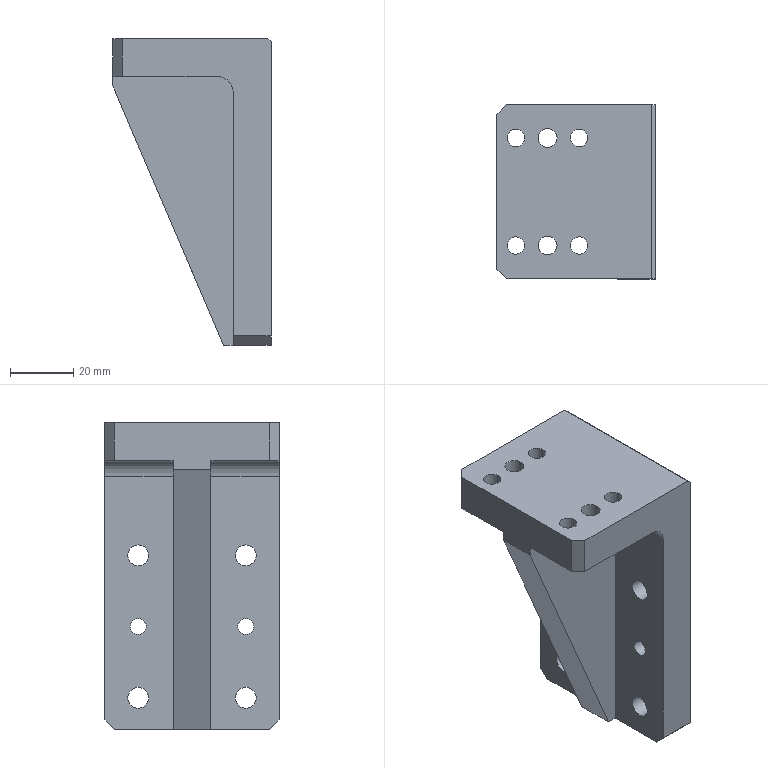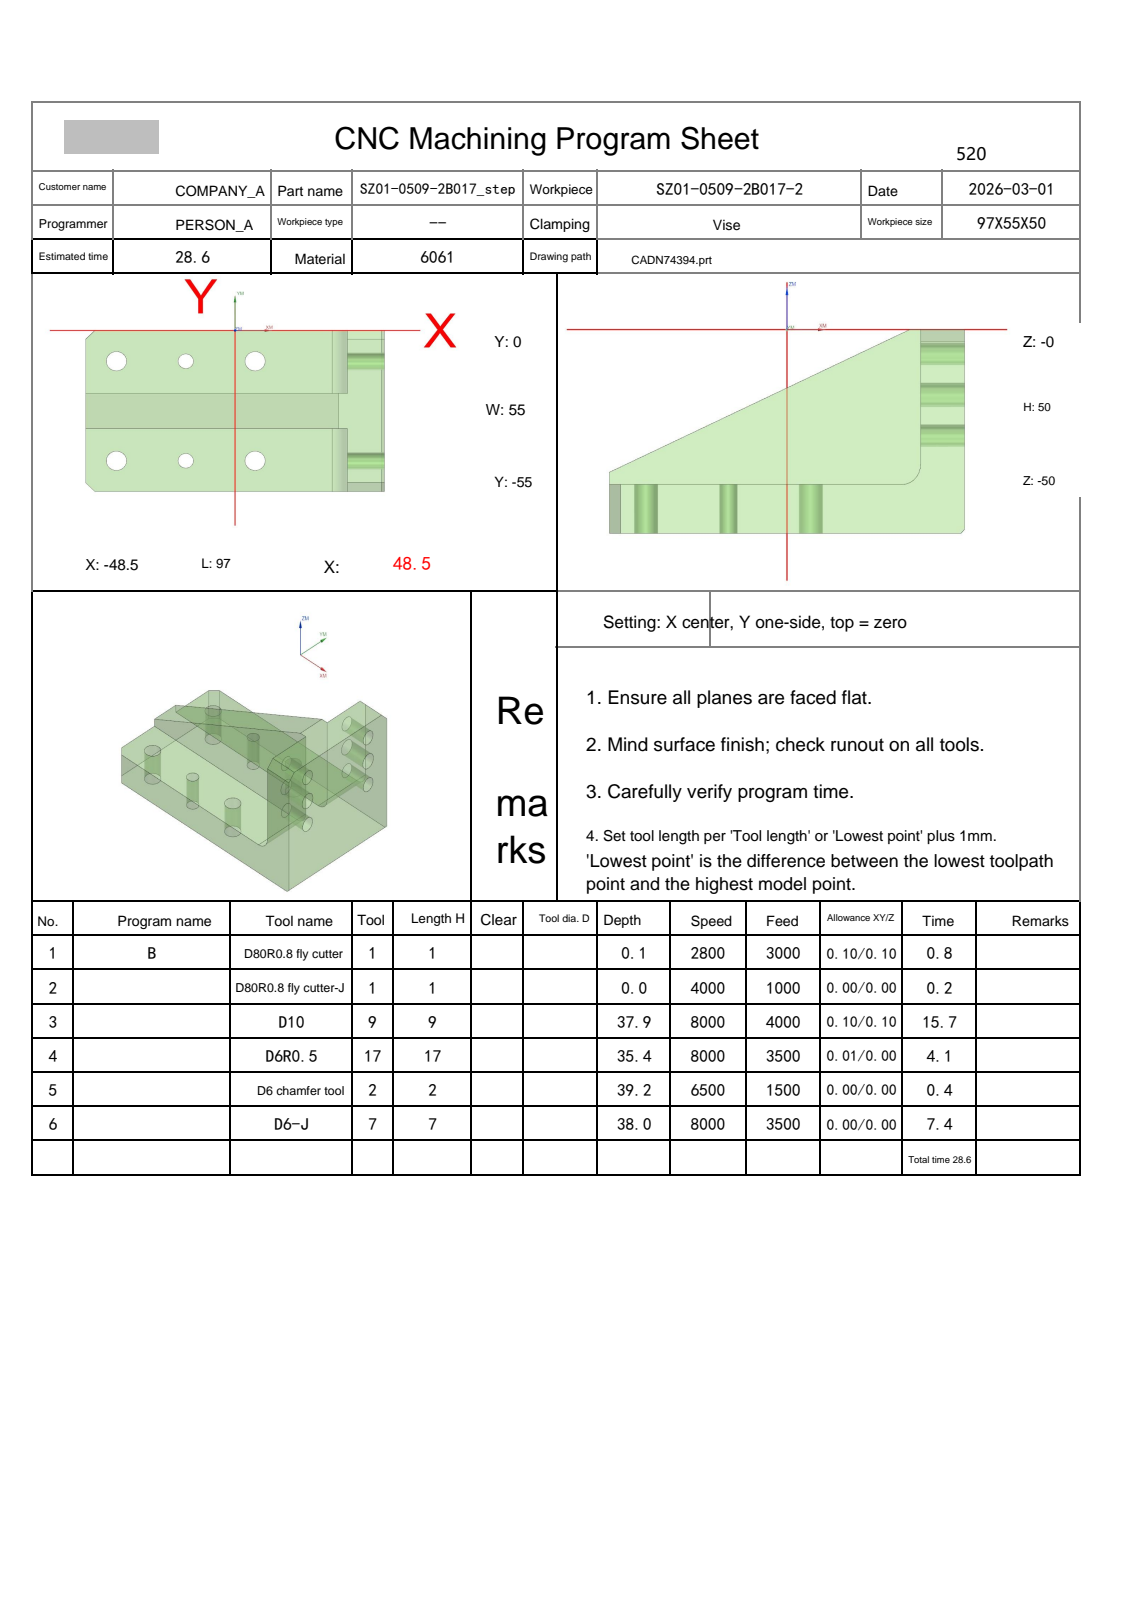NC program | NX | posted by the shop | part box 50 x 55 x 97 mm
Lines 110 to 1246 of 18128:
N3 T09 M06
(D10  D=10. R=0. H=09 ce=0.10 di=0.10)
G00 G90 G54 X-4.751 Y-69.5 M03 S8000
G43 H09 Z14.5
M08
Z.701
G01 Z-.499 F4000.
Y-62.08
G03 X-11.751 Y-55.08 I-7. J0.0
G01 X-45.5
X-45.557 Y-55.057
X-48.557 Y-52.057
X-48.58 Y-52.
Y-38.678
G02 X-50.965 Y-38.008 I.232 J5.41
X-51.5 Y-37.642 I2.818 J4.689
G01 Y-17.385
G02 X-48.58 Y-16.325 I3.189 J-4.232
G01 Y-3.
X-48.557 Y-2.943
X-45.557 Y.057
X-45.5 Y.08
X31.301
X31.324 Y.09
X31.362 Y.651
G02 X32.353 Y3. I5.275 J-.842
G01 X32.988
G02 X36.5 Y4.04 I3.533 J-5.481
G01 X48.42
Y3.
X48.5
X48.504 Y4.04
X48.501 Y3.
X48.58
Y2.64
X48.501
X48.5 Y2.641
X48.499 Y2.64
X48.42 Y2.641
X36.5 Y2.64
G03 X31.424 Y-1.987 I.021 J-5.121
G01 X31.379 Y-2.26
X31.344 Y-2.498
X31.321 Y-2.991
X31.32 Y-3.243
X31.321 Y-3.438
X31.32 Y-16.494
G03 X27.077 Y-21.5 I.856 J-5.027
G01 Y-33.5
G03 X31.322 Y-38.506 I5.1 J.022
G01 X31.321 Y-51.562
Y-52.069
X31.345 Y-52.51
X31.424 Y-53.011
G03 X36.5 Y-57.64 I5.097 J.491
G01 X48.42
X48.499
X48.5 Y-57.641
X48.501 Y-57.64
X48.58
Y-58.
X48.502
X48.506 Y-59.04
X48.5
Y-58.
X48.42
Y-59.04
X36.494
G02 X32.988 Y-58. I.026 J6.521
G01 X32.301
G02 X31.32 Y-55.082 I4.155 J3.02
G01 X30.524 Y-55.081
X26.802 Y-55.08
X25.909
X-8.737
G02 X-9.55 Y-54.662 I.001 J1.
G01 X-13.952 Y-48.498
G03 X-14.765 Y-48.08 I-.813 J-.582
G01 X-40.582
G02 X-41.58 Y-47.082 I.002 J1.
G01 Y-38.678
G03 X-44.136 Y-33.269 I-7. J0.0
G02 X-44.5 Y-32.5 I.636 J.771
G01 Y-22.503
G02 X-44.136 Y-21.734 I1. J-.002
G03 X-41.58 Y-16.325 I-4.444 J5.409
G01 Y-7.918
G02 X-40.582 Y-6.92 I1. J-.002
G01 X23.323
G02 X24.321 Y-7.918 I-.002 J-1.
G01 Y-11.871
G02 X23.998 Y-12.605 I-1. J.002
G03 X20.077 Y-21.485 I8.179 J-8.917
G01 Y-33.515
G03 X23.999 Y-42.396 I12.1 J.037
G02 X24.322 Y-43.13 I-.677 J-.736
G01 Y-47.082
G02 X23.324 Y-48.08 I-1. J.002
G01 X-8.737
G02 X-9.55 Y-47.662 I0.0 J1.
G01 X-13.952 Y-41.498
G03 X-14.765 Y-41.08 I-.814 J-.582
G01 X-33.582
G02 X-34.58 Y-40.082 I.002 J1.
G01 Y-38.678
G03 X-37.307 Y-30.376 I-14. J0.0
G02 X-37.5 Y-29.788 I.807 J.591
G01 Y-25.215
G02 X-37.307 Y-24.626 I1. J-.002
G03 X-34.58 Y-16.325 I-11.273 J8.301
G01 Y-14.918
G02 X-33.582 Y-13.92 I1. J-.002
G01 X13.194
G02 X14.192 Y-14.92 I-.002 J-1.
X14.137 Y-15.247 I-1. J0.0
G03 X13.077 Y-21.474 I18.039 J-6.275
G01 Y-33.526
G03 X14.137 Y-39.754 I19.1 J.047
G02 X14.192 Y-40.08 I-.945 J-.326
X13.194 Y-41.08 I-1. J0.0
G01 X-8.737
G02 X-9.55 Y-40.662 I0.0 J1.
G01 X-13.952 Y-34.498
G03 X-14.765 Y-34.08 I-.814 J-.582
G01 X-27.307
G02 X-28.27 Y-33.337 I.003 J1.
G03 X-30.368 Y-28.221 I-20.31 J-5.341
G02 X-30.5 Y-27.728 I.869 J.496
G01 Y-27.275
G02 X-30.368 Y-26.782 I1. J-.003
G03 X-28.27 Y-21.663 I-18.212 J10.457
G02 X-27.306 Y-20.92 I.966 J-.257
G01 X5.08
G02 X6.077 Y-21.918 I-.003 J-1.
G01 Y-33.083
G02 X5.08 Y-34.08 I-1. J.003
G01 X-9.087
G02 X-9.794 Y-33.787 I0.0 J1.
G01 X-13.708 Y-29.873
G03 X-14.415 Y-29.58 I-.707 J-.707
G01 X-24.082
G02 X-25.003 Y-28.964 I.003 J1.
G03 X-25.46 Y-27.921 I-23.577 J-9.714
G02 X-25.552 Y-27.501 I.908 J.419
X-25.46 Y-27.082 I1. J0.0
G03 X-25.002 Y-26.037 I-23.12 J10.757
G02 X-24.081 Y-25.42 I.924 J-.383
G01 X.58
G02 X1.577 Y-26.417 I-.003 J-1.
G01 Y-28.583
G02 X.58 Y-29.58 I-1. J.003
G01 X-11.751
X-12.251
G03 X-19.251 Y-36.58 I0.0 J-7.
G01 Z.701
G00 Z3.
G01 X-4.751 Y-69.5 F6000.
G00 Z.203
G01 Z-.997 F4000.
Y-62.08
G03 X-11.751 Y-55.08 I-7. J0.0
G01 X-45.5
X-45.557 Y-55.057
X-48.557 Y-52.057
X-48.58 Y-52.
Y-38.678
G02 X-50.965 Y-38.008 I.232 J5.41
X-53.609 Y-33.631 I2.818 J4.689
G01 Y-21.36
X-53.545 Y-20.788
G02 X-48.58 Y-16.325 I5.234 J-.83
G01 Y-3.
X-48.557 Y-2.943
X-45.557 Y.057
X-45.5 Y.08
X31.301
X31.324 Y.09
X31.362 Y.651
G02 X36.629 Y5.151 I5.275 J-.842
G01 X48.501
X48.585 Y5.156
X48.581 Y5.071
X48.58 Y3.139
X48.5
X48.42
X36.5
G03 X31.398 Y-1.984 I.021 J-5.122
G01 X31.4 Y-2.119
X31.344 Y-2.498
X31.321 Y-2.991
X31.32 Y-3.243
X31.321 Y-3.438
X31.32 Y-16.4
X31.163
X31.09 Y-16.399
G03 X25.909 Y-21.5 I0.0 J-5.183
G01 Y-33.5
G03 X31.09 Y-38.601 I5.182 J.082
G01 X31.163 Y-38.6
X31.322
X31.321 Y-51.562
Y-52.069
X31.345 Y-52.51
X31.4 Y-52.879
Y-52.997
Y-53.018
G03 X36.5 Y-58.139 I5.121 J0.0
G01 X48.42
X48.5
X48.58
X48.581 Y-60.071
X48.585 Y-60.156
X48.501 Y-60.151
X36.623 Y-60.15
X35.717 Y-60.071
X34.817 Y-59.849
G02 X31.32 Y-55.082 I1.639 J4.868
G01 X26.802 Y-55.08
X25.909
X-8.737
G02 X-9.55 Y-54.662 I.001 J1.
G01 X-13.952 Y-48.498
G03 X-14.765 Y-48.08 I-.813 J-.582
G01 X-40.582
G02 X-41.58 Y-47.082 I.002 J1.
G01 Y-38.678
G03 X-45.982 Y-32.178 I-7. J0.0
G02 X-46.609 Y-31.251 I.373 J.928
G01 Y-23.751
G02 X-45.982 Y-22.825 I1. J-.002
G03 X-41.58 Y-16.325 I-2.598 J6.5
G01 Y-7.918
G02 X-40.582 Y-6.92 I1. J-.002
G01 X23.322
G02 X24.321 Y-7.919 I-.002 J-1.
G01 Y-10.934
G02 X23.911 Y-11.74 I-1. J.002
G03 X18.909 Y-21.445 I7.179 J-9.842
G01 Y-33.555
G03 X23.912 Y-43.261 I12.182 J.138
G02 X24.322 Y-44.067 I-.591 J-.807
G01 Y-47.082
G02 X23.323 Y-48.08 I-1. J.002
G01 X-8.737
G02 X-9.55 Y-47.662 I0.0 J1.
G01 X-13.952 Y-41.498
G03 X-14.765 Y-41.08 I-.814 J-.582
G01 X-33.582
G02 X-34.58 Y-40.082 I.002 J1.
G01 Y-38.678
G03 X-39.244 Y-28.245 I-14. J0.0
G02 X-39.576 Y-27.501 I.668 J.744
X-39.244 Y-26.757 I1. J0.0
G03 X-34.58 Y-16.325 I-9.336 J10.433
G01 Y-14.918
G02 X-33.582 Y-13.92 I1. J-.002
G01 X12.041
G02 X13.039 Y-14.92 I-.002 J-1.
X12.984 Y-15.249 I-1. J0.0
G03 X11.909 Y-21.365 I18.107 J-6.334
G01 Y-33.634
G03 X12.984 Y-39.752 I19.181 J.217
G02 X13.039 Y-40.08 I-.945 J-.328
X12.041 Y-41.08 I-1. J0.0
G01 X-8.737
G02 X-9.55 Y-40.662 I0.0 J1.
G01 X-13.952 Y-34.498
G03 X-14.765 Y-34.08 I-.814 J-.582
G01 X-27.306
G02 X-28.271 Y-33.337 I.002 J1.
G03 X-30.493 Y-28.007 I-20.309 J-5.341
G02 X-30.63 Y-27.501 I.863 J.506
X-30.493 Y-26.995 I1. J0.0
G03 X-28.27 Y-21.664 I-18.087 J10.67
G02 X-27.306 Y-20.92 I.967 J-.257
G01 X3.911
G02 X4.909 Y-21.918 I-.002 J-1.
G01 Y-33.082
G02 X3.911 Y-34.08 I-1. J.002
G01 X-9.087
G02 X-9.794 Y-33.787 I0.0 J1.
G01 X-13.708 Y-29.873
G03 X-14.415 Y-29.58 I-.707 J-.707
G01 X-24.082
G02 X-25.003 Y-28.963 I.003 J1.
G03 X-25.46 Y-27.921 I-23.577 J-9.714
G02 X-25.552 Y-27.501 I.908 J.419
X-25.46 Y-27.082 I1. J0.0
G03 X-25.002 Y-26.037 I-23.12 J10.757
G02 X-24.081 Y-25.42 I.924 J-.383
G01 X-.588
G02 X.409 Y-26.418 I-.003 J-1.
G01 Y-28.583
G02 X-.588 Y-29.58 I-1. J.003
G01 X-11.751
X-12.251
G03 X-19.251 Y-36.58 I0.0 J-7.
G01 Z.203
G00 Z3.
G01 X-4.751 Y-69.5 F6000.
G00 Z-.296
G01 Z-1.496 F4000.
Y-62.08
G03 X-11.751 Y-55.08 I-7. J0.0
G01 X-45.5
X-45.557 Y-55.057
X-48.557 Y-52.057
X-48.58 Y-52.
Y-38.678
G02 X-50.965 Y-38.008 I.232 J5.41
X-53.609 Y-33.631 I2.818 J4.689
G01 Y-21.36
X-53.545 Y-20.788
G02 X-48.58 Y-16.325 I5.234 J-.83
G01 Y-3.
X-48.557 Y-2.943
X-45.557 Y.057
X-45.5 Y.08
X31.301
X31.324 Y.09
X31.362 Y.651
G02 X36.629 Y5.151 I5.275 J-.842
G01 X48.501
X48.585 Y5.156
X48.581 Y5.071
X48.58 Y3.637
X48.5
X48.42
X36.5
G03 X31.4 Y-1.483 I.021 J-5.121
G01 Y-1.504
Y-2.119
X31.344 Y-2.498
X31.321 Y-2.991
X31.32 Y-3.243
X31.321 Y-3.438
X31.32 Y-16.4
X29.995
X29.925
G03 X24.74 Y-21.5 I0.0 J-5.185
G01 Y-33.5
G03 X29.925 Y-38.6 I5.185 J.085
G01 X29.995
X31.018
X31.163
X31.322
X31.321 Y-51.562
Y-52.069
X31.345 Y-52.51
X31.4 Y-52.879
Y-53.496
Y-53.517
G03 X36.5 Y-58.637 I5.121 J0.0
G01 X48.42
X48.499
X48.58
X48.581 Y-60.071
X48.585 Y-60.156
X48.501 Y-60.151
X36.623 Y-60.15
X35.717 Y-60.071
X34.817 Y-59.849
G02 X31.32 Y-55.082 I1.639 J4.868
G01 X26.802 Y-55.08
X25.909
X-8.737
G02 X-9.55 Y-54.662 I0.0 J1.
G01 X-13.952 Y-48.498
G03 X-14.765 Y-48.08 I-.813 J-.582
G01 X-40.582
G02 X-41.58 Y-47.082 I.002 J1.
G01 Y-38.678
G03 X-45.982 Y-32.178 I-7. J0.0
G02 X-46.609 Y-31.251 I.373 J.928
G01 Y-23.751
G02 X-45.982 Y-22.825 I1. J-.002
G03 X-41.58 Y-16.325 I-2.598 J6.5
G01 Y-7.918
G02 X-40.582 Y-6.92 I1. J-.002
G01 X23.323
G02 X24.321 Y-7.919 I-.002 J-1.
G01 Y-10.175
G02 X23.823 Y-11.037 I-1. J.002
G03 X17.74 Y-21.443 I6.102 J-10.548
G01 Y-33.557
G03 X23.824 Y-43.963 I12.185 J.143
G02 X24.322 Y-44.826 I-.502 J-.865
G01 Y-47.082
G02 X23.323 Y-48.08 I-1. J.002
G01 X-8.737
G02 X-9.55 Y-47.662 I0.0 J1.
G01 X-13.952 Y-41.498
G03 X-14.765 Y-41.08 I-.814 J-.582
G01 X-33.582
G02 X-34.58 Y-40.082 I.002 J1.
G01 Y-38.678
G03 X-39.244 Y-28.245 I-14. J0.0
G02 X-39.576 Y-27.501 I.668 J.744
X-39.244 Y-26.758 I1. J0.0
G03 X-34.58 Y-16.325 I-9.336 J10.433
G01 Y-14.918
G02 X-33.582 Y-13.92 I1. J-.002
G01 X10.874
G02 X11.871 Y-14.92 I-.002 J-1.
X11.816 Y-15.249 I-1. J0.0
G03 X10.74 Y-21.402 I18.109 J-6.337
G01 Y-33.598
G03 X11.816 Y-39.752 I19.185 J.184
G02 X11.872 Y-40.08 I-.945 J-.328
X10.874 Y-41.08 I-1. J0.0
G01 X-8.737
G02 X-9.55 Y-40.662 I0.0 J1.
G01 X-13.952 Y-34.498
G03 X-14.765 Y-34.08 I-.814 J-.582
G01 X-27.306
G02 X-28.271 Y-33.337 I.002 J1.
G03 X-30.493 Y-28.007 I-20.309 J-5.341
G02 X-30.63 Y-27.501 I.863 J.506
X-30.493 Y-26.995 I1. J0.0
G03 X-28.27 Y-21.663 I-18.087 J10.67
G02 X-27.306 Y-20.92 I.967 J-.257
G01 X2.743
G02 X3.74 Y-21.918 I-.002 J-1.
G01 Y-33.082
G02 X2.743 Y-34.08 I-1. J.002
G01 X-9.087
G02 X-9.794 Y-33.787 I0.0 J1.
G01 X-13.708 Y-29.873
G03 X-14.415 Y-29.58 I-.707 J-.707
G01 X-24.082
G02 X-25.003 Y-28.963 I.003 J1.
G03 X-25.46 Y-27.921 I-23.577 J-9.714
G02 X-25.552 Y-27.501 I.908 J.419
X-25.46 Y-27.082 I1. J0.0
G03 X-25.002 Y-26.037 I-23.12 J10.757
G02 X-24.081 Y-25.42 I.924 J-.383
G01 X-1.757
G02 X-.76 Y-26.418 I-.003 J-1.
G01 Y-28.583
G02 X-1.757 Y-29.58 I-1. J.003
G01 X-11.751
X-12.251
G03 X-19.251 Y-36.58 I0.0 J-7.
G01 Z-.296
G00 Z3.
G01 X-4.751 Y-69.5 F6000.
G00 Z-.795
G01 Z-1.995 F4000.
Y-62.08
G03 X-11.751 Y-55.08 I-7. J0.0
G01 X-45.5
X-45.557 Y-55.057
X-48.557 Y-52.057
X-48.58 Y-52.
Y-38.678
G02 X-50.965 Y-38.008 I.232 J5.41
X-53.609 Y-33.631 I2.818 J4.689
G01 Y-21.36
X-53.545 Y-20.788
G02 X-48.58 Y-16.325 I5.234 J-.83
G01 Y-3.
X-48.557 Y-2.943
X-45.557 Y.057
X-45.5 Y.08
X31.301
X31.324 Y.09
X31.362 Y.651
G02 X36.629 Y5.151 I5.275 J-.842
G01 X48.501
X48.585 Y5.156
X48.581 Y5.071
X48.58 Y4.136
X48.5
X48.496
X48.42
X36.5
G03 X31.4 Y-.985 I.021 J-5.121
G01 Y-1.005
Y-2.119
X31.344 Y-2.498
X31.321 Y-2.991
X31.32 Y-3.243
X31.321 Y-3.438
X31.32 Y-16.4
X29.995
X29.855
X28.827
X28.749 Y-16.399
G03 X23.572 Y-21.5 I0.0 J-5.178
G01 Y-33.5
G03 X28.749 Y-38.601 I5.177 J.077
G01 X28.827 Y-38.6
X31.322
X31.321 Y-51.562
Y-52.069
X31.345 Y-52.51
X31.4 Y-52.879
Y-53.995
Y-54.015
G03 X36.5 Y-59.136 I5.121 J0.0
G01 X48.42
X48.496
X48.5
X48.58
X48.581 Y-60.071
X48.585 Y-60.156
X48.501 Y-60.151
X36.623 Y-60.15
X35.717 Y-60.071
X34.817 Y-59.849
G02 X31.32 Y-55.082 I1.639 J4.868
G01 X26.802 Y-55.08
X25.909
X-8.737
G02 X-9.55 Y-54.662 I.001 J1.
G01 X-13.952 Y-48.498
G03 X-14.765 Y-48.08 I-.813 J-.582
G01 X-40.582
G02 X-41.58 Y-47.082 I.002 J1.
G01 Y-38.678
G03 X-45.982 Y-32.178 I-7. J0.0
G02 X-46.609 Y-31.252 I.373 J.928
G01 Y-23.751
G02 X-45.982 Y-22.825 I1. J-.002
G03 X-41.58 Y-16.325 I-2.598 J6.5
G01 Y-7.918
G02 X-40.582 Y-6.92 I1. J-.002
G01 X23.323
G02 X24.321 Y-7.919 I-.002 J-1.
G01 Y-9.571
G02 X23.734 Y-10.48 I-1. J.002
G03 X16.572 Y-21.448 I5.015 J-11.097
G01 Y-33.552
G03 X23.735 Y-44.52 I12.177 J.13
G02 X24.322 Y-45.429 I-.414 J-.91
G01 Y-47.082
G02 X23.323 Y-48.08 I-1. J.002
G01 X-8.737
G02 X-9.55 Y-47.662 I0.0 J1.
G01 X-13.952 Y-41.498
G03 X-14.765 Y-41.08 I-.813 J-.582
G01 X-33.582
G02 X-34.58 Y-40.082 I.002 J1.
G01 Y-38.678
G03 X-39.244 Y-28.245 I-14. J0.0
G02 X-39.576 Y-27.501 I.669 J.744
X-39.244 Y-26.758 I1. J0.0
G03 X-34.58 Y-16.325 I-9.336 J10.433
G01 Y-14.918
G02 X-33.582 Y-13.92 I1. J-.002
G01 X9.703
G02 X10.701 Y-14.92 I-.002 J-1.
X10.646 Y-15.248 I-1. J0.0
G03 X9.572 Y-21.373 I18.103 J-6.329
G01 Y-33.627
G03 X10.646 Y-39.752 I19.177 J.204
G02 X10.701 Y-40.08 I-.945 J-.328
X9.703 Y-41.08 I-1. J0.0
G01 X-8.737
G02 X-9.55 Y-40.662 I0.0 J1.
G01 X-13.952 Y-34.498
G03 X-14.765 Y-34.08 I-.814 J-.582
G01 X-27.307
G02 X-28.271 Y-33.337 I.003 J1.
G03 X-30.493 Y-28.007 I-20.309 J-5.341
G02 X-30.63 Y-27.501 I.863 J.506
X-30.493 Y-26.995 I1. J0.0
G03 X-28.27 Y-21.663 I-18.087 J10.671
G02 X-27.306 Y-20.92 I.966 J-.257
G01 X1.575
G02 X2.572 Y-21.918 I-.003 J-1.
G01 Y-33.083
G02 X1.575 Y-34.08 I-1. J.003
G01 X-9.087
G02 X-9.794 Y-33.787 I0.0 J1.
G01 X-13.708 Y-29.873
G03 X-14.415 Y-29.58 I-.707 J-.707
G01 X-24.082
G02 X-25.003 Y-28.963 I.003 J1.
G03 X-25.46 Y-27.921 I-23.577 J-9.714
G02 X-25.552 Y-27.501 I.908 J.419
X-25.46 Y-27.082 I1. J0.0
G03 X-25.002 Y-26.037 I-23.12 J10.757
G02 X-24.081 Y-25.42 I.924 J-.383
G01 X-2.925
G02 X-1.928 Y-26.418 I-.003 J-1.
G01 Y-28.583
G02 X-2.925 Y-29.58 I-1. J.003
G01 X-11.751
X-12.251
G03 X-19.251 Y-36.58 I0.0 J-7.
G01 Z-.795
G00 Z3.
G01 X-4.751 Y-69.5 F6000.
G00 Z-1.293
G01 Z-2.493 F4000.
Y-62.08
G03 X-11.751 Y-55.08 I-7. J0.0
G01 X-45.5
X-45.557 Y-55.057
X-48.557 Y-52.057
X-48.58 Y-52.
Y-38.678
G02 X-50.965 Y-38.008 I.232 J5.41
X-53.609 Y-33.631 I2.818 J4.689
G01 Y-21.36
X-53.545 Y-20.788
G02 X-48.58 Y-16.325 I5.234 J-.83
G01 Y-3.
X-48.557 Y-2.943
X-45.557 Y.057
X-45.5 Y.08
X31.301
X31.324 Y.09
X31.362 Y.651
G02 X36.629 Y5.151 I5.275 J-.842
G01 X48.501
X48.585 Y5.156
X48.581 Y5.071
X48.58 Y4.635
X48.5
X48.491
X48.42
X36.5
G03 X31.4 Y-.486 I.021 J-5.121
G01 Y-.507
Y-2.119
X31.344 Y-2.498
X31.321 Y-2.991
X31.32 Y-3.243
X31.321 Y-3.438
X31.32 Y-16.4
X27.658
X27.581 Y-16.399
G03 X22.404 Y-21.5 I0.0 J-5.178
G01 Y-33.5
G03 X27.581 Y-38.601 I5.177 J.077
G01 X27.658 Y-38.6
X28.672
X28.827
X31.322
X31.321 Y-51.562
Y-52.069
X31.345 Y-52.51
X31.4 Y-52.879
Y-54.493
Y-54.514
G03 X36.5 Y-59.635 I5.121 J0.0
G01 X48.42
X48.483
X48.5
X48.58
X48.581 Y-60.071
X48.585 Y-60.156
X48.501 Y-60.151
X36.623 Y-60.15
X35.717 Y-60.071
X34.817 Y-59.849
G02 X31.32 Y-55.082 I1.639 J4.868
G01 X26.802 Y-55.08
X25.909
X-8.737
G02 X-9.55 Y-54.662 I0.0 J1.
G01 X-13.952 Y-48.498
G03 X-14.765 Y-48.08 I-.813 J-.582
G01 X-40.582
G02 X-41.58 Y-47.082 I.002 J1.
G01 Y-38.678
G03 X-45.982 Y-32.178 I-7. J0.0
G02 X-46.609 Y-31.252 I.373 J.928
G01 Y-23.751
G02 X-45.982 Y-22.825 I1. J-.002
G03 X-41.58 Y-16.325 I-2.598 J6.5
G01 Y-7.918
G02 X-40.582 Y-6.92 I1. J-.002
G01 X23.323
G02 X24.321 Y-7.918 I-.002 J-1.
G01 Y-9.109
G02 X23.646 Y-10.053 I-1. J.002
G03 X15.404 Y-21.448 I3.935 J-11.525
G01 Y-33.605
G03 X23.647 Y-44.948 I12.177 J.182
G02 X24.322 Y-45.891 I-.325 J-.946
G01 Y-47.082
G02 X23.324 Y-48.08 I-1. J.002
G01 X-8.737
G02 X-9.55 Y-47.662 I0.0 J1.
G01 X-13.952 Y-41.498
G03 X-14.765 Y-41.08 I-.814 J-.582
G01 X-33.582
G02 X-34.58 Y-40.082 I.002 J1.
G01 Y-38.678
G03 X-39.244 Y-28.245 I-14. J0.0
G02 X-39.576 Y-27.501 I.669 J.744
X-39.244 Y-26.758 I1. J0.0
G03 X-34.58 Y-16.325 I-9.336 J10.433
G01 Y-14.918
G02 X-33.582 Y-13.92 I1. J-.002
G01 X8.535
G02 X9.533 Y-14.92 I-.002 J-1.
X9.477 Y-15.248 I-1. J0.0
G03 X8.404 Y-21.411 I18.103 J-6.33
G01 X8.405 Y-33.709
G03 X9.478 Y-39.752 I19.176 J.287
G02 X9.533 Y-40.08 I-.945 J-.328
X8.535 Y-41.08 I-1. J0.0
G01 X-8.737
G02 X-9.55 Y-40.662 I0.0 J1.
G01 X-13.952 Y-34.498
G03 X-14.765 Y-34.08 I-.814 J-.582
G01 X-27.307
G02 X-28.27 Y-33.337 I.003 J1.
G03 X-30.493 Y-28.007 I-20.31 J-5.341
G02 X-30.63 Y-27.501 I.863 J.506
X-30.493 Y-26.996 I1. J0.0
G03 X-28.27 Y-21.663 I-18.087 J10.671
G02 X-27.306 Y-20.92 I.966 J-.257
G01 X.406
G02 X1.404 Y-21.917 I-.003 J-1.
G01 X1.405 Y-33.083
G02 X.408 Y-34.08 I-1. J.003
G01 X-9.087
G02 X-9.794 Y-33.787 I0.0 J1.
G01 X-13.708 Y-29.873
G03 X-14.415 Y-29.58 I-.707 J-.707
G01 X-24.082
G02 X-25.003 Y-28.964 I.003 J1.
G03 X-25.46 Y-27.921 I-23.577 J-9.714
G02 X-25.552 Y-27.501 I.908 J.419
X-25.46 Y-27.082 I1. J0.0
G03 X-25.002 Y-26.037 I-23.12 J10.757
G02 X-24.081 Y-25.42 I.924 J-.383
G01 X-4.093
G02 X-3.096 Y-26.417 I-.003 J-1.
G01 Y-28.583
G02 X-4.093 Y-29.58 I-1. J.003
G01 X-11.751
X-12.251
G03 X-19.251 Y-36.58 I0.0 J-7.
G01 Z-1.293
G00 Z3.
G01 X-4.751 Y-69.5 F6000.
G00 Z-1.792
G01 Z-2.992 F4000.
Y-62.08
G03 X-11.751 Y-55.08 I-7. J0.0
G01 X-45.5
X-45.557 Y-55.057
X-48.557 Y-52.057
X-48.58 Y-52.
Y-38.678
G02 X-50.965 Y-38.008 I.232 J5.41
X-51.5 Y-37.642 I2.818 J4.689
G01 Y-17.385
G02 X-48.58 Y-16.325 I3.189 J-4.232
G01 Y-3.
X-48.557 Y-2.943
X-45.557 Y.057
X-45.5 Y.08
X31.301
X31.324 Y.09
X31.368 Y.688
X31.454 Y.673
G03 X31.4 Y.005 I4.076 J-.668
G01 Y-.008
Y-2.119
X31.344 Y-2.498
X31.321 Y-2.991
X31.32 Y-3.243
X31.321 Y-3.438
X31.32 Y-16.4
X27.658
X27.504
X26.49
X26.432
G03 X21.235 Y-21.5 I0.0 J-5.198
G01 Y-33.5
G03 X26.432 Y-38.6 I5.197 J.097
G01 X26.49
X31.322
Y-40.
X31.321 Y-51.562
Y-52.069
X31.345 Y-52.51
X31.4 Y-52.879
Y-54.992
Y-55.005
G03 X31.454 Y-55.673 I4.13 J0.0
G01 X31.368 Y-55.685
G02 X31.32 Y-55.082 I5.088 J.705
G01 X26.802 Y-55.08
X25.909
X-8.737
G02 X-9.55 Y-54.662 I0.0 J1.
G01 X-13.952 Y-48.498
G03 X-14.765 Y-48.08 I-.813 J-.582
G01 X-40.583
G02 X-41.58 Y-47.083 I.003 J1.
G01 Y-38.678
G03 X-44.137 Y-33.269 I-7. J0.0
G02 X-44.5 Y-32.5 I.637 J.771
G01 Y-22.502
G02 X-44.137 Y-21.734 I1. J-.003
G03 X-41.58 Y-16.325 I-4.443 J5.409
G01 Y-7.917
G02 X-40.583 Y-6.92 I1. J-.003
G01 X23.324
G02 X24.321 Y-7.918 I-.003 J-1.
G01 Y-8.774
G02 X23.559 Y-9.743 I-1. J.003
G03 X14.235 Y-21.434 I2.873 J-11.855
G01 Y-33.566
G03 X23.56 Y-45.257 I12.197 J.163
G02 X24.322 Y-46.226 I-.238 J-.971
G01 Y-47.083
G02 X23.324 Y-48.08 I-1. J.003
G01 X-8.737
G02 X-9.55 Y-47.662 I0.0 J1.
G01 X-13.952 Y-41.498
G03 X-14.765 Y-41.08 I-.814 J-.582
G01 X-33.583
G02 X-34.58 Y-40.083 I.003 J1.
G01 Y-38.678
G03 X-37.307 Y-30.376 I-14. J0.0
G02 X-37.5 Y-29.788 I.807 J.591
G01 Y-25.214
G02 X-37.307 Y-24.627 I1. J-.003
G03 X-34.58 Y-16.325 I-11.273 J8.302
G01 Y-14.917
G02 X-33.583 Y-13.92 I1. J-.003
G01 X7.373
G02 X8.37 Y-14.92 I-.003 J-1.
X8.314 Y-15.248 I-1. J0.0
G03 X7.235 Y-21.388 I18.117 J-6.349
G01 Y-33.612
G03 X8.315 Y-39.752 I19.197 J.21
G02 X8.37 Y-40.08 I-.945 J-.328
X7.373 Y-41.08 I-1. J0.0
G01 X-8.737
G02 X-9.55 Y-40.662 I0.0 J1.
G01 X-13.952 Y-34.498
G03 X-14.765 Y-34.08 I-.814 J-.582
G01 X-27.307
G02 X-28.27 Y-33.337 I.003 J1.
G03 X-30.369 Y-28.221 I-20.31 J-5.34
G02 X-30.5 Y-27.729 I.869 J.495
G01 Y-27.274
G02 X-30.369 Y-26.782 I1. J-.003
G03 X-28.27 Y-21.663 I-18.211 J10.457
G02 X-27.307 Y-20.92 I.966 J-.257
G01 X-.762
G02 X.235 Y-21.917 I-.003 J-1.
G01 Y-33.083
G02 X-.762 Y-34.08 I-1. J.003
G01 X-9.087
G02 X-9.794 Y-33.787 I0.0 J1.
G01 X-13.708 Y-29.873
G03 X-14.415 Y-29.58 I-.707 J-.707
G01 X-24.083
G02 X-25.003 Y-28.964 I.003 J1.
G03 X-25.46 Y-27.92 I-23.577 J-9.714
G02 X-25.552 Y-27.501 I.908 J.419
X-25.46 Y-27.082 I1. J0.0
G03 X-25.002 Y-26.036 I-23.12 J10.758
G02 X-24.081 Y-25.42 I.923 J-.384
G01 X-5.262
G02 X-4.265 Y-26.417 I-.003 J-1.
G01 Y-28.583
G02 X-5.262 Y-29.58 I-1. J.003
G01 X-11.751
X-12.251
G03 X-19.251 Y-36.58 I0.0 J-7.
G01 Z-1.792
G00 Z3.
G01 X-4.751 Y-69.5 F6000.
G00 Z-2.291
G01 Z-3.491 F4000.
Y-62.08
G03 X-11.751 Y-55.08 I-7. J0.0
G01 X-45.5
X-45.557 Y-55.057
X-48.557 Y-52.057
X-48.58 Y-52.
Y-38.678
G02 X-50.965 Y-38.008 I.232 J5.41
X-51.5 Y-37.642 I2.818 J4.689
G01 Y-17.385
G02 X-48.58 Y-16.325 I3.189 J-4.232
G01 Y-3.
X-48.557 Y-2.943
X-45.557 Y.057
X-45.5 Y.08
X31.301
X31.324 Y.09
X31.4 Y-.013
Y-2.119
X31.344 Y-2.498
X31.321 Y-2.991
X31.32 Y-3.243
X31.321 Y-3.438
X31.32 Y-16.4
X27.658
X27.504
X25.322
X25.244 Y-16.399
G03 X20.067 Y-21.5 I0.0 J-5.178
G01 Y-33.5
G03 X25.244 Y-38.601 I5.177 J.077
G01 X25.322 Y-38.6
X31.322
Y-40.
X31.321 Y-51.562
Y-52.069
X31.345 Y-52.51
X31.4 Y-52.879
Y-55.039
X31.32 Y-55.082
X26.802 Y-55.08
X25.909
X-8.737
G02 X-9.55 Y-54.662 I0.0 J1.
G01 X-13.952 Y-48.498
G03 X-14.765 Y-48.08 I-.813 J-.582
G01 X-40.583
G02 X-41.58 Y-47.083 I.003 J1.
G01 Y-38.678
G03 X-44.137 Y-33.269 I-7. J0.0
G02 X-44.5 Y-32.5 I.637 J.771
G01 Y-22.502
G02 X-44.137 Y-21.734 I1. J-.003
G03 X-41.58 Y-16.325 I-4.443 J5.409
G01 Y-7.917
G02 X-40.583 Y-6.92 I1. J-.003
G01 X23.324
G02 X24.321 Y-7.918 I-.003 J-1.
G01 Y-8.543
G02 X23.469 Y-9.529 I-1. J.003
G03 X13.067 Y-21.448 I1.775 J-12.048
G01 Y-33.552
G03 X23.47 Y-45.471 I12.177 J.13
G02 X24.322 Y-46.457 I-.148 J-.989
G01 Y-47.083
G02 X23.324 Y-48.08 I-1. J.003
G01 X-8.737
G02 X-9.55 Y-47.662 I0.0 J1.
G01 X-13.952 Y-41.498
G03 X-14.765 Y-41.08 I-.814 J-.582
G01 X-33.583
G02 X-34.58 Y-40.083 I.003 J1.
G01 Y-38.678
G03 X-37.307 Y-30.376 I-14. J0.0
G02 X-37.5 Y-29.788 I.807 J.59
G01 Y-25.214
G02 X-37.307 Y-24.627 I1. J-.003
G03 X-34.58 Y-16.325 I-11.273 J8.302
G01 Y-14.917
G02 X-33.583 Y-13.92 I1. J-.003
G01 X6.199
G02 X7.196 Y-14.92 I-.003 J-1.
X7.141 Y-15.247 I-1. J0.0
G03 X6.067 Y-21.41 I18.103 J-6.33
G01 Y-33.59
G03 X7.141 Y-39.753 I19.177 J.167
G02 X7.196 Y-40.08 I-.945 J-.327
X6.199 Y-41.08 I-1. J0.0
G01 X-8.737
G02 X-9.55 Y-40.662 I0.0 J1.
G01 X-13.952 Y-34.498
G03 X-14.765 Y-34.08 I-.814 J-.582
G01 X-27.307
G02 X-28.27 Y-33.337 I.003 J1.
G03 X-30.369 Y-28.221 I-20.31 J-5.34
G02 X-30.5 Y-27.729 I.869 J.495
G01 Y-27.274
G02 X-30.369 Y-26.782 I1. J-.003
G03 X-28.27 Y-21.663 I-18.211 J10.457
G02 X-27.307 Y-20.92 I.966 J-.257
G01 X-1.93
G02 X-.933 Y-21.917 I-.003 J-1.
G01 Y-33.083
G02 X-1.93 Y-34.08 I-1. J.003
G01 X-9.087
G02 X-9.794 Y-33.787 I0.0 J1.
G01 X-13.708 Y-29.873
G03 X-14.415 Y-29.58 I-.707 J-.707
G01 X-24.083
G02 X-25.003 Y-28.964 I.003 J1.
G03 X-25.46 Y-27.92 I-23.577 J-9.714
G02 X-25.552 Y-27.501 I.908 J.419
X-25.46 Y-27.082 I1. J0.0
G03 X-25.002 Y-26.036 I-23.12 J10.758
G02 X-24.082 Y-25.42 I.923 J-.384
G01 X-6.43
G02 X-5.433 Y-26.417 I-.003 J-1.
G01 Y-28.583
G02 X-6.43 Y-29.58 I-1. J.003
G01 X-11.751
X-12.251
G03 X-19.251 Y-36.58 I0.0 J-7.
G01 Z-2.291
G00 Z3.
G01 X-4.751 Y-69.5 F6000.
G00 Z-2.789
G01 Z-3.989 F4000.
Y-62.08
G03 X-11.751 Y-55.08 I-7. J0.0
G01 X-45.5
X-45.557 Y-55.057
X-48.557 Y-52.057
X-48.58 Y-52.
Y-38.678
G02 X-50.965 Y-38.008 I.232 J5.41
X-51.5 Y-37.642 I2.818 J4.689
G01 Y-17.385
G02 X-48.58 Y-16.325 I3.189 J-4.232
G01 Y-3.
X-48.557 Y-2.943
X-45.557 Y.057
X-45.5 Y.08
X31.301
X31.324 Y.09
X31.4 Y-.013
Y-2.119
X31.374 Y-2.292
X31.344 Y-2.498
X31.321 Y-2.991
X31.32 Y-3.243
X31.321 Y-3.438
X31.32 Y-16.4
X24.153
X24.076 Y-16.399
G03 X18.898 Y-21.5 I0.0 J-5.178
G01 X18.9 Y-33.555
G03 X24.076 Y-38.601 I5.176 J.133
G01 X24.153 Y-38.6
X25.167
X25.322
X31.322
X31.321 Y-51.562
Y-52.069
X31.345 Y-52.51
X31.4 Y-52.879
Y-55.038
X31.32 Y-55.082
X26.802 Y-55.08
X25.909
X-8.737
G02 X-9.55 Y-54.662 I0.0 J1.
G01 X-13.952 Y-48.498
G03 X-14.765 Y-48.08 I-.813 J-.582
G01 X-40.583
G02 X-41.58 Y-47.083 I.003 J1.
G01 Y-38.678
G03 X-44.137 Y-33.268 I-7. J0.0
G02 X-44.5 Y-32.5 I.637 J.771
G01 Y-22.502
G02 X-44.137 Y-21.734 I1. J-.003
G03 X-41.58 Y-16.325 I-4.443 J5.409
G01 Y-7.917
G02 X-40.583 Y-6.92 I1. J-.003
G01 X23.324
G02 X24.321 Y-7.918 I-.003 J-1.
G01 Y-8.424
G02 X23.381 Y-9.419 I-1. J.003
G03 X11.898 Y-21.448 I.695 J-12.158
G01 X11.899 Y-33.605
G03 X23.382 Y-45.581 I12.177 J.182
G02 X24.322 Y-46.576 I-.06 J-.998
G01 Y-47.083
G02 X23.324 Y-48.08 I-1. J.003
G01 X-8.737
G02 X-9.55 Y-47.662 I0.0 J1.
G01 X-13.952 Y-41.498
G03 X-14.765 Y-41.08 I-.814 J-.582
G01 X-33.583
G02 X-34.58 Y-40.083 I.003 J1.
G01 Y-38.678
G03 X-37.307 Y-30.376 I-14. J0.0
G02 X-37.5 Y-29.789 I.807 J.59
G01 Y-25.214
G02 X-37.307 Y-24.627 I1. J-.003
G03 X-34.58 Y-16.325 I-11.273 J8.302
G01 Y-14.917
G02 X-33.583 Y-13.92 I1. J-.003
G01 X5.031
G02 X6.028 Y-14.92 I-.003 J-1.
X5.973 Y-15.247 I-1. J0.0
G03 X4.898 Y-21.41 I18.103 J-6.33
G01 Y-33.605
G03 X5.973 Y-39.753 I19.177 J.183
G02 X6.028 Y-40.08 I-.945 J-.327
X5.031 Y-41.08 I-1. J0.0
G01 X-8.737
G02 X-9.55 Y-40.662 I0.0 J1.
G01 X-13.952 Y-34.498
G03 X-14.765 Y-34.08 I-.814 J-.582
G01 X-27.307
G02 X-28.27 Y-33.338 I.003 J1.
G03 X-30.369 Y-28.221 I-20.31 J-5.34
G02 X-30.5 Y-27.729 I.869 J.495
G01 Y-27.274
G02 X-30.369 Y-26.782 I1. J-.003
G03 X-28.27 Y-21.663 I-18.211 J10.457
G02 X-27.307 Y-20.92 I.966 J-.257
G01 X-3.098
G02 X-2.102 Y-21.917 I-.003 J-1.
G01 Y-33.083
G02 X-3.098 Y-34.08 I-1. J.003
G01 X-9.087
G02 X-9.794 Y-33.787 I0.0 J1.
G01 X-13.708 Y-29.873
G03 X-14.415 Y-29.58 I-.707 J-.707
G01 X-24.083
G02 X-25.003 Y-28.964 I.003 J1.
G03 X-25.46 Y-27.92 I-23.577 J-9.714
G02 X-25.552 Y-27.501 I.908 J.419
X-25.46 Y-27.083 I1. J0.0
G03 X-25.002 Y-26.036 I-23.12 J10.758
G02 X-24.082 Y-25.42 I.923 J-.384
G01 X-7.598
G02 X-6.602 Y-26.417 I-.003 J-1.
G01 Y-28.583
G02 X-7.598 Y-29.58 I-1. J.003
G01 X-11.751
X-12.251
G03 X-19.251 Y-36.58 I0.0 J-7.
G01 Z-2.789
G00 Z3.
G01 X-4.751 Y-69.5 F6000.
G00 Z-3.288
G01 Z-4.488 F4000.
Y-62.08
G03 X-11.751 Y-55.08 I-7. J0.0
G01 X-45.5
X-45.557 Y-55.057
X-48.557 Y-52.057
X-48.58 Y-52.